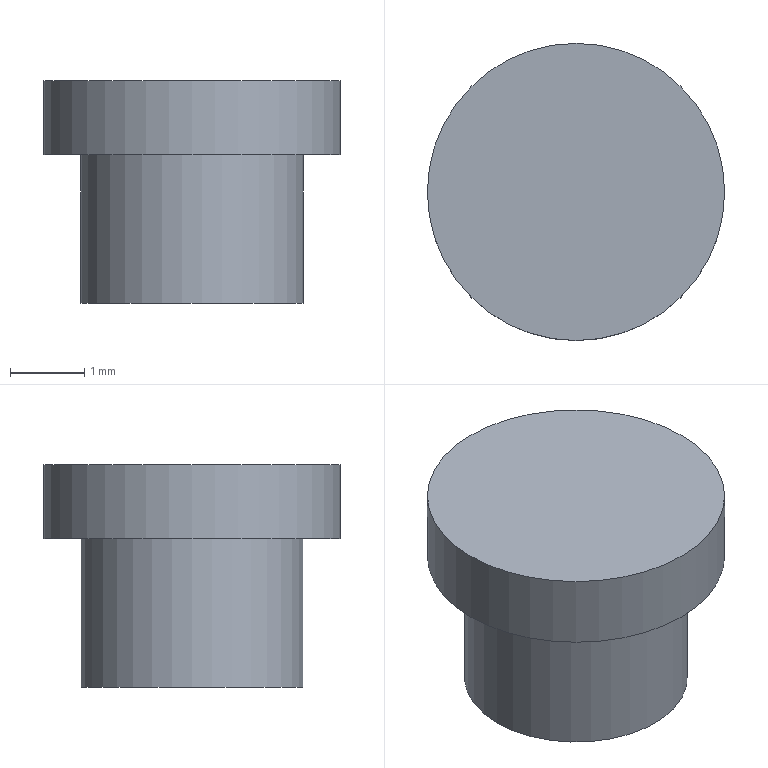Part | NX | features CYLINDER 2, DATUM_CSYS 1 | 1 solid | 5 faces | box 4 x 4 x 3 mm | volume 26.704 mm3 | plane 3 | cylinder 2 | commonest cylinder face diameters 3 x1 4 x1
STEP:
#1=CARTESIAN_POINT('',(1.5,0.,0.));
#2=VERTEX_POINT('',#1);
#3=CARTESIAN_POINT('',(0.,0.,0.));
#4=DIRECTION('',(0.,0.,1.));
#5=DIRECTION('',(1.,0.,0.));
#6=AXIS2_PLACEMENT_3D('',#3,#4,#5);
#7=CIRCLE('',#6,1.5);
#8=EDGE_CURVE('',#2,#2,#7,.T.);
#9=ORIENTED_EDGE('',*,*,#8,.F.);
#10=EDGE_LOOP('',(#9));
#11=FACE_BOUND('',#10,.T.);
#12=CARTESIAN_POINT('',(0.,0.,0.));
#13=DIRECTION('',(0.,0.,-1.));
#14=DIRECTION('',(-1.,0.,0.));
#15=AXIS2_PLACEMENT_3D('',#12,#13,#14);
#16=PLANE('',#15);
#17=ADVANCED_FACE('',(#11),#16,.T.);
#18=CARTESIAN_POINT('',(1.5,0.,2.));
#19=VERTEX_POINT('',#18);
#20=CARTESIAN_POINT('',(0.,0.,2.));
#21=DIRECTION('',(0.,0.,-1.));
#22=DIRECTION('',(1.,0.,0.));
#23=AXIS2_PLACEMENT_3D('',#20,#21,#22);
#24=CIRCLE('',#23,1.5);
#25=EDGE_CURVE('',#19,#19,#24,.T.);
#26=ORIENTED_EDGE('',*,*,#25,.T.);
#27=EDGE_LOOP('',(#26));
#28=FACE_BOUND('',#27,.T.);
#29=ORIENTED_EDGE('',*,*,#8,.T.);
#30=EDGE_LOOP('',(#29));
#31=FACE_BOUND('',#30,.T.);
#32=CARTESIAN_POINT('',(0.,0.,0.));
#33=DIRECTION('',(0.,0.,1.));
#34=DIRECTION('',(1.,0.,0.));
#35=AXIS2_PLACEMENT_3D('',#32,#33,#34);
#36=CYLINDRICAL_SURFACE('',#35,1.5);
#37=ADVANCED_FACE('',(#28,#31),#36,.T.);
#38=CARTESIAN_POINT('',(2.,0.,3.));
#39=VERTEX_POINT('',#38);
#40=CARTESIAN_POINT('',(0.,0.,3.));
#41=DIRECTION('',(0.,0.,-1.));
#42=DIRECTION('',(1.,0.,0.));
#43=AXIS2_PLACEMENT_3D('',#40,#41,#42);
#44=CIRCLE('',#43,2.);
#45=EDGE_CURVE('',#39,#39,#44,.T.);
#46=ORIENTED_EDGE('',*,*,#45,.F.);
#47=EDGE_LOOP('',(#46));
#48=FACE_BOUND('',#47,.T.);
#49=CARTESIAN_POINT('',(0.,0.,3.));
#50=DIRECTION('',(0.,0.,1.));
#51=DIRECTION('',(1.,0.,0.));
#52=AXIS2_PLACEMENT_3D('',#49,#50,#51);
#53=PLANE('',#52);
#54=ADVANCED_FACE('',(#48),#53,.T.);
#55=ORIENTED_EDGE('',*,*,#25,.F.);
#56=EDGE_LOOP('',(#55));
#57=FACE_BOUND('',#56,.T.);
#58=CARTESIAN_POINT('',(2.,0.,2.));
#59=VERTEX_POINT('',#58);
#60=CARTESIAN_POINT('',(0.,0.,2.));
#61=DIRECTION('',(0.,0.,1.));
#62=DIRECTION('',(1.,0.,0.));
#63=AXIS2_PLACEMENT_3D('',#60,#61,#62);
#64=CIRCLE('',#63,2.);
#65=EDGE_CURVE('',#59,#59,#64,.T.);
#66=ORIENTED_EDGE('',*,*,#65,.F.);
#67=EDGE_LOOP('',(#66));
#68=FACE_BOUND('',#67,.T.);
#69=CARTESIAN_POINT('',(0.,0.,2.));
#70=DIRECTION('',(0.,0.,-1.));
#71=DIRECTION('',(-1.,0.,0.));
#72=AXIS2_PLACEMENT_3D('',#69,#70,#71);
#73=PLANE('',#72);
#74=ADVANCED_FACE('',(#57,#68),#73,.T.);
#75=ORIENTED_EDGE('',*,*,#45,.T.);
#76=EDGE_LOOP('',(#75));
#77=FACE_BOUND('',#76,.T.);
#78=ORIENTED_EDGE('',*,*,#65,.T.);
#79=EDGE_LOOP('',(#78));
#80=FACE_BOUND('',#79,.T.);
#81=CARTESIAN_POINT('',(0.,0.,2.));
#82=DIRECTION('',(0.,0.,1.));
#83=DIRECTION('',(1.,0.,0.));
#84=AXIS2_PLACEMENT_3D('',#81,#82,#83);
#85=CYLINDRICAL_SURFACE('',#84,2.);
#86=ADVANCED_FACE('',(#77,#80),#85,.T.);
#87=CLOSED_SHELL('',(#17,#37,#54,#74,#86));
#88=MANIFOLD_SOLID_BREP('',#87);
#89=(LENGTH_UNIT()NAMED_UNIT(*)SI_UNIT(.MILLI.,.METRE.));
#90=UNCERTAINTY_MEASURE_WITH_UNIT(LENGTH_MEASURE(0.00001),#89,'','');
#91=(NAMED_UNIT(*)PLANE_ANGLE_UNIT()SI_UNIT($,.RADIAN.));
#92=(NAMED_UNIT(*)SI_UNIT($,.STERADIAN.)SOLID_ANGLE_UNIT());
#93=(GEOMETRIC_REPRESENTATION_CONTEXT(3)GLOBAL_UNCERTAINTY_ASSIGNED_CONTEXT((#90))GLOBAL_UNIT_ASSIGNED_CONTEXT((#89,#91,#92))REPRESENTATION_CONTEXT('',''));
#94=ADVANCED_BREP_SHAPE_REPRESENTATION('',(#88),#93);